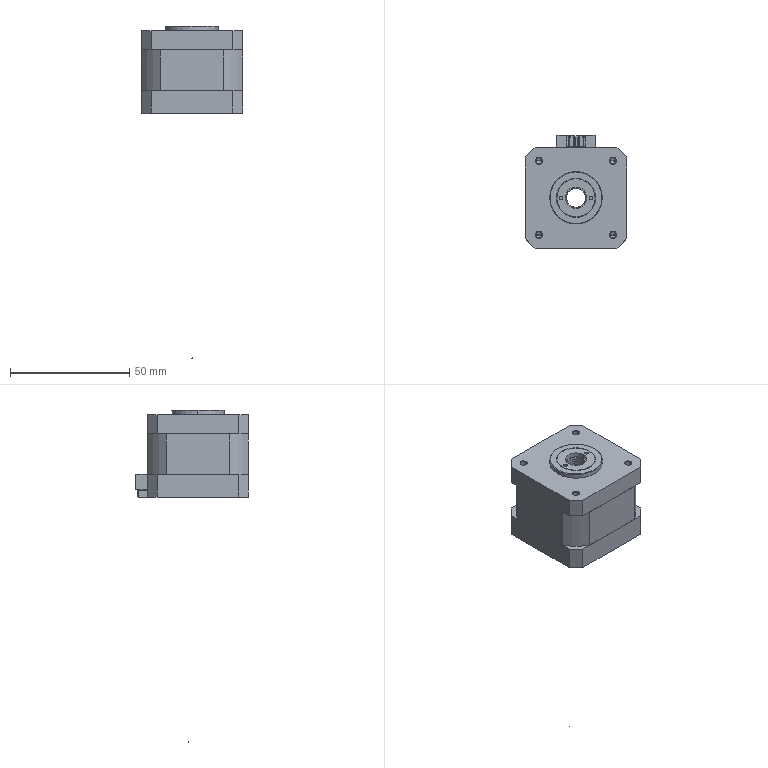Part | STEP file | 42HSC1409-250NE2V1.201001 | 2 solids | 530 faces | box 42.3 x 47.3 x 139 mm | volume 58209 mm3 | plane 296 | cylinder 100 | spline 95 | cone 39 | commonest cylinder face diameters 8 x35 2.5 x16 0.8 x12 6.5 x8 48 x8 1.5 x4